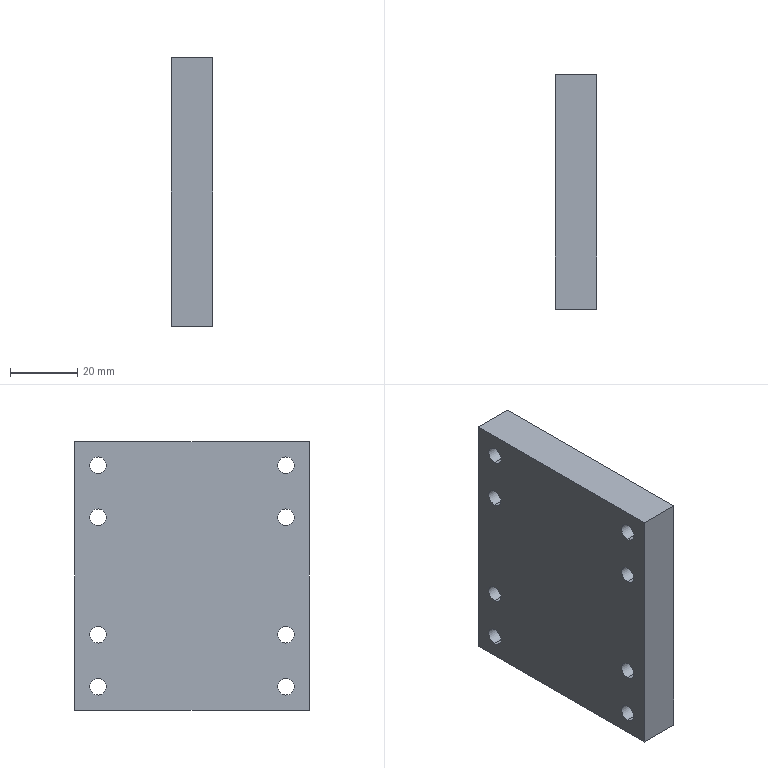Part | SolidWorks | features HoleWzd 2, Extrusion 1 | 1 solid | 22 faces | box 12.4 x 70 x 80 mm | volume 67492 mm3 | cylinder 16 | plane 6 | commonest cylinder face diameters 5 x16
STEP:
#1=CARTESIAN_POINT('',(0.,28.,35.5));
#2=VERTEX_POINT('',#1);
#3=CARTESIAN_POINT('',(0.,28.,30.5));
#4=VERTEX_POINT('',#3);
#5=CARTESIAN_POINT('',(0.,28.,33.));
#6=DIRECTION('',(1.,0.,0.));
#7=DIRECTION('',(0.,0.,-1.));
#8=AXIS2_PLACEMENT_3D('',#5,#6,#7);
#9=CIRCLE('',#8,2.5);
#10=EDGE_CURVE('',#2,#4,#9,.T.);
#11=ORIENTED_EDGE('',*,*,#10,.F.);
#12=CARTESIAN_POINT('',(12.4,28.,35.5));
#13=VERTEX_POINT('',#12);
#14=CARTESIAN_POINT('',(12.4,28.,35.5));
#15=DIRECTION('',(1.,0.,0.));
#16=VECTOR('',#15,1000.);
#17=LINE('',#14,#16);
#18=EDGE_CURVE('',#2,#13,#17,.T.);
#19=ORIENTED_EDGE('',*,*,#18,.T.);
#20=CARTESIAN_POINT('',(12.4,28.,30.5));
#21=VERTEX_POINT('',#20);
#22=CARTESIAN_POINT('',(12.4,28.,33.));
#23=DIRECTION('',(1.,0.,0.));
#24=DIRECTION('',(0.,0.,-1.));
#25=AXIS2_PLACEMENT_3D('',#22,#23,#24);
#26=CIRCLE('',#25,2.5);
#27=EDGE_CURVE('',#13,#21,#26,.T.);
#28=ORIENTED_EDGE('',*,*,#27,.T.);
#29=CARTESIAN_POINT('',(12.4,28.,30.5));
#30=DIRECTION('',(1.,0.,0.));
#31=VECTOR('',#30,1000.);
#32=LINE('',#29,#31);
#33=EDGE_CURVE('',#4,#21,#32,.T.);
#34=ORIENTED_EDGE('',*,*,#33,.F.);
#35=EDGE_LOOP('',(#11,#19,#28,#34));
#36=FACE_OUTER_BOUND('',#35,.T.);
#37=CARTESIAN_POINT('',(12.4,28.,33.));
#38=DIRECTION('',(1.,0.,0.));
#39=DIRECTION('',(0.,0.,-1.));
#40=AXIS2_PLACEMENT_3D('',#37,#38,#39);
#41=CYLINDRICAL_SURFACE('',#40,2.5);
#42=ADVANCED_FACE('',(#36),#41,.F.);
#43=CARTESIAN_POINT('',(0.,-28.,35.5));
#44=VERTEX_POINT('',#43);
#45=CARTESIAN_POINT('',(0.,-28.,30.5));
#46=VERTEX_POINT('',#45);
#47=CARTESIAN_POINT('',(0.,-28.,33.));
#48=DIRECTION('',(1.,0.,0.));
#49=DIRECTION('',(0.,0.,-1.));
#50=AXIS2_PLACEMENT_3D('',#47,#48,#49);
#51=CIRCLE('',#50,2.5);
#52=EDGE_CURVE('',#44,#46,#51,.T.);
#53=ORIENTED_EDGE('',*,*,#52,.F.);
#54=CARTESIAN_POINT('',(12.4,-28.,35.5));
#55=VERTEX_POINT('',#54);
#56=CARTESIAN_POINT('',(12.4,-28.,35.5));
#57=DIRECTION('',(1.,0.,0.));
#58=VECTOR('',#57,1000.);
#59=LINE('',#56,#58);
#60=EDGE_CURVE('',#44,#55,#59,.T.);
#61=ORIENTED_EDGE('',*,*,#60,.T.);
#62=CARTESIAN_POINT('',(12.4,-28.,30.5));
#63=VERTEX_POINT('',#62);
#64=CARTESIAN_POINT('',(12.4,-28.,33.));
#65=DIRECTION('',(1.,0.,0.));
#66=DIRECTION('',(0.,0.,-1.));
#67=AXIS2_PLACEMENT_3D('',#64,#65,#66);
#68=CIRCLE('',#67,2.5);
#69=EDGE_CURVE('',#55,#63,#68,.T.);
#70=ORIENTED_EDGE('',*,*,#69,.T.);
#71=CARTESIAN_POINT('',(12.4,-28.,30.5));
#72=DIRECTION('',(1.,0.,0.));
#73=VECTOR('',#72,1000.);
#74=LINE('',#71,#73);
#75=EDGE_CURVE('',#46,#63,#74,.T.);
#76=ORIENTED_EDGE('',*,*,#75,.F.);
#77=EDGE_LOOP('',(#53,#61,#70,#76));
#78=FACE_OUTER_BOUND('',#77,.T.);
#79=CARTESIAN_POINT('',(12.4,-28.,33.));
#80=DIRECTION('',(1.,0.,0.));
#81=DIRECTION('',(0.,0.,-1.));
#82=AXIS2_PLACEMENT_3D('',#79,#80,#81);
#83=CYLINDRICAL_SURFACE('',#82,2.5);
#84=ADVANCED_FACE('',(#78),#83,.F.);
#85=CARTESIAN_POINT('',(0.,-28.,-30.5));
#86=VERTEX_POINT('',#85);
#87=CARTESIAN_POINT('',(0.,-28.,-35.5));
#88=VERTEX_POINT('',#87);
#89=CARTESIAN_POINT('',(0.,-28.,-33.));
#90=DIRECTION('',(1.,0.,0.));
#91=DIRECTION('',(0.,0.,-1.));
#92=AXIS2_PLACEMENT_3D('',#89,#90,#91);
#93=CIRCLE('',#92,2.5);
#94=EDGE_CURVE('',#86,#88,#93,.T.);
#95=ORIENTED_EDGE('',*,*,#94,.F.);
#96=CARTESIAN_POINT('',(12.4,-28.,-30.5));
#97=VERTEX_POINT('',#96);
#98=CARTESIAN_POINT('',(12.4,-28.,-30.5));
#99=DIRECTION('',(1.,0.,0.));
#100=VECTOR('',#99,1000.);
#101=LINE('',#98,#100);
#102=EDGE_CURVE('',#86,#97,#101,.T.);
#103=ORIENTED_EDGE('',*,*,#102,.T.);
#104=CARTESIAN_POINT('',(12.4,-28.,-35.5));
#105=VERTEX_POINT('',#104);
#106=CARTESIAN_POINT('',(12.4,-28.,-33.));
#107=DIRECTION('',(1.,0.,0.));
#108=DIRECTION('',(0.,0.,-1.));
#109=AXIS2_PLACEMENT_3D('',#106,#107,#108);
#110=CIRCLE('',#109,2.5);
#111=EDGE_CURVE('',#97,#105,#110,.T.);
#112=ORIENTED_EDGE('',*,*,#111,.T.);
#113=CARTESIAN_POINT('',(12.4,-28.,-35.5));
#114=DIRECTION('',(1.,0.,0.));
#115=VECTOR('',#114,1000.);
#116=LINE('',#113,#115);
#117=EDGE_CURVE('',#88,#105,#116,.T.);
#118=ORIENTED_EDGE('',*,*,#117,.F.);
#119=EDGE_LOOP('',(#95,#103,#112,#118));
#120=FACE_OUTER_BOUND('',#119,.T.);
#121=CARTESIAN_POINT('',(12.4,-28.,-33.));
#122=DIRECTION('',(1.,0.,0.));
#123=DIRECTION('',(0.,0.,-1.));
#124=AXIS2_PLACEMENT_3D('',#121,#122,#123);
#125=CYLINDRICAL_SURFACE('',#124,2.5);
#126=ADVANCED_FACE('',(#120),#125,.F.);
#127=CARTESIAN_POINT('',(0.,28.,-30.5));
#128=VERTEX_POINT('',#127);
#129=CARTESIAN_POINT('',(0.,28.,-35.5));
#130=VERTEX_POINT('',#129);
#131=CARTESIAN_POINT('',(0.,28.,-33.));
#132=DIRECTION('',(1.,0.,0.));
#133=DIRECTION('',(0.,0.,-1.));
#134=AXIS2_PLACEMENT_3D('',#131,#132,#133);
#135=CIRCLE('',#134,2.5);
#136=EDGE_CURVE('',#128,#130,#135,.T.);
#137=ORIENTED_EDGE('',*,*,#136,.F.);
#138=CARTESIAN_POINT('',(12.4,28.,-30.5));
#139=VERTEX_POINT('',#138);
#140=CARTESIAN_POINT('',(12.4,28.,-30.5));
#141=DIRECTION('',(1.,0.,0.));
#142=VECTOR('',#141,1000.);
#143=LINE('',#140,#142);
#144=EDGE_CURVE('',#128,#139,#143,.T.);
#145=ORIENTED_EDGE('',*,*,#144,.T.);
#146=CARTESIAN_POINT('',(12.4,28.,-35.5));
#147=VERTEX_POINT('',#146);
#148=CARTESIAN_POINT('',(12.4,28.,-33.));
#149=DIRECTION('',(1.,0.,0.));
#150=DIRECTION('',(0.,0.,-1.));
#151=AXIS2_PLACEMENT_3D('',#148,#149,#150);
#152=CIRCLE('',#151,2.5);
#153=EDGE_CURVE('',#139,#147,#152,.T.);
#154=ORIENTED_EDGE('',*,*,#153,.T.);
#155=CARTESIAN_POINT('',(12.4,28.,-35.5));
#156=DIRECTION('',(1.,0.,0.));
#157=VECTOR('',#156,1000.);
#158=LINE('',#155,#157);
#159=EDGE_CURVE('',#130,#147,#158,.T.);
#160=ORIENTED_EDGE('',*,*,#159,.F.);
#161=EDGE_LOOP('',(#137,#145,#154,#160));
#162=FACE_OUTER_BOUND('',#161,.T.);
#163=CARTESIAN_POINT('',(12.4,28.,-33.));
#164=DIRECTION('',(1.,0.,0.));
#165=DIRECTION('',(0.,0.,-1.));
#166=AXIS2_PLACEMENT_3D('',#163,#164,#165);
#167=CYLINDRICAL_SURFACE('',#166,2.5);
#168=ADVANCED_FACE('',(#162),#167,.F.);
#169=CARTESIAN_POINT('',(0.,28.,20.));
#170=VERTEX_POINT('',#169);
#171=CARTESIAN_POINT('',(0.,28.,15.));
#172=VERTEX_POINT('',#171);
#173=CARTESIAN_POINT('',(0.,28.,17.5));
#174=DIRECTION('',(1.,0.,0.));
#175=DIRECTION('',(0.,0.,-1.));
#176=AXIS2_PLACEMENT_3D('',#173,#174,#175);
#177=CIRCLE('',#176,2.5);
#178=EDGE_CURVE('',#170,#172,#177,.T.);
#179=ORIENTED_EDGE('',*,*,#178,.F.);
#180=CARTESIAN_POINT('',(12.4,28.,20.));
#181=VERTEX_POINT('',#180);
#182=CARTESIAN_POINT('',(12.4,28.,20.));
#183=DIRECTION('',(1.,0.,0.));
#184=VECTOR('',#183,1000.);
#185=LINE('',#182,#184);
#186=EDGE_CURVE('',#170,#181,#185,.T.);
#187=ORIENTED_EDGE('',*,*,#186,.T.);
#188=CARTESIAN_POINT('',(12.4,28.,15.));
#189=VERTEX_POINT('',#188);
#190=CARTESIAN_POINT('',(12.4,28.,17.5));
#191=DIRECTION('',(1.,0.,0.));
#192=DIRECTION('',(0.,0.,-1.));
#193=AXIS2_PLACEMENT_3D('',#190,#191,#192);
#194=CIRCLE('',#193,2.5);
#195=EDGE_CURVE('',#181,#189,#194,.T.);
#196=ORIENTED_EDGE('',*,*,#195,.T.);
#197=CARTESIAN_POINT('',(12.4,28.,15.));
#198=DIRECTION('',(1.,0.,0.));
#199=VECTOR('',#198,1000.);
#200=LINE('',#197,#199);
#201=EDGE_CURVE('',#172,#189,#200,.T.);
#202=ORIENTED_EDGE('',*,*,#201,.F.);
#203=EDGE_LOOP('',(#179,#187,#196,#202));
#204=FACE_OUTER_BOUND('',#203,.T.);
#205=CARTESIAN_POINT('',(12.4,28.,17.5));
#206=DIRECTION('',(1.,0.,0.));
#207=DIRECTION('',(0.,0.,-1.));
#208=AXIS2_PLACEMENT_3D('',#205,#206,#207);
#209=CYLINDRICAL_SURFACE('',#208,2.5);
#210=ADVANCED_FACE('',(#204),#209,.F.);
#211=CARTESIAN_POINT('',(0.,28.,-15.));
#212=VERTEX_POINT('',#211);
#213=CARTESIAN_POINT('',(0.,28.,-20.));
#214=VERTEX_POINT('',#213);
#215=CARTESIAN_POINT('',(0.,28.,-17.5));
#216=DIRECTION('',(1.,0.,0.));
#217=DIRECTION('',(0.,0.,-1.));
#218=AXIS2_PLACEMENT_3D('',#215,#216,#217);
#219=CIRCLE('',#218,2.5);
#220=EDGE_CURVE('',#212,#214,#219,.T.);
#221=ORIENTED_EDGE('',*,*,#220,.F.);
#222=CARTESIAN_POINT('',(12.4,28.,-15.));
#223=VERTEX_POINT('',#222);
#224=CARTESIAN_POINT('',(12.4,28.,-15.));
#225=DIRECTION('',(1.,0.,0.));
#226=VECTOR('',#225,1000.);
#227=LINE('',#224,#226);
#228=EDGE_CURVE('',#212,#223,#227,.T.);
#229=ORIENTED_EDGE('',*,*,#228,.T.);
#230=CARTESIAN_POINT('',(12.4,28.,-20.));
#231=VERTEX_POINT('',#230);
#232=CARTESIAN_POINT('',(12.4,28.,-17.5));
#233=DIRECTION('',(1.,0.,0.));
#234=DIRECTION('',(0.,0.,-1.));
#235=AXIS2_PLACEMENT_3D('',#232,#233,#234);
#236=CIRCLE('',#235,2.5);
#237=EDGE_CURVE('',#223,#231,#236,.T.);
#238=ORIENTED_EDGE('',*,*,#237,.T.);
#239=CARTESIAN_POINT('',(12.4,28.,-20.));
#240=DIRECTION('',(1.,0.,0.));
#241=VECTOR('',#240,1000.);
#242=LINE('',#239,#241);
#243=EDGE_CURVE('',#214,#231,#242,.T.);
#244=ORIENTED_EDGE('',*,*,#243,.F.);
#245=EDGE_LOOP('',(#221,#229,#238,#244));
#246=FACE_OUTER_BOUND('',#245,.T.);
#247=CARTESIAN_POINT('',(12.4,28.,-17.5));
#248=DIRECTION('',(1.,0.,0.));
#249=DIRECTION('',(0.,0.,-1.));
#250=AXIS2_PLACEMENT_3D('',#247,#248,#249);
#251=CYLINDRICAL_SURFACE('',#250,2.5);
#252=ADVANCED_FACE('',(#246),#251,.F.);
#253=CARTESIAN_POINT('',(0.,-28.,20.));
#254=VERTEX_POINT('',#253);
#255=CARTESIAN_POINT('',(0.,-28.,15.));
#256=VERTEX_POINT('',#255);
#257=CARTESIAN_POINT('',(0.,-28.,17.5));
#258=DIRECTION('',(1.,0.,0.));
#259=DIRECTION('',(0.,0.,-1.));
#260=AXIS2_PLACEMENT_3D('',#257,#258,#259);
#261=CIRCLE('',#260,2.5);
#262=EDGE_CURVE('',#254,#256,#261,.T.);
#263=ORIENTED_EDGE('',*,*,#262,.F.);
#264=CARTESIAN_POINT('',(12.4,-28.,20.));
#265=VERTEX_POINT('',#264);
#266=CARTESIAN_POINT('',(12.4,-28.,20.));
#267=DIRECTION('',(1.,0.,0.));
#268=VECTOR('',#267,1000.);
#269=LINE('',#266,#268);
#270=EDGE_CURVE('',#254,#265,#269,.T.);
#271=ORIENTED_EDGE('',*,*,#270,.T.);
#272=CARTESIAN_POINT('',(12.4,-28.,15.));
#273=VERTEX_POINT('',#272);
#274=CARTESIAN_POINT('',(12.4,-28.,17.5));
#275=DIRECTION('',(1.,0.,0.));
#276=DIRECTION('',(0.,0.,-1.));
#277=AXIS2_PLACEMENT_3D('',#274,#275,#276);
#278=CIRCLE('',#277,2.5);
#279=EDGE_CURVE('',#265,#273,#278,.T.);
#280=ORIENTED_EDGE('',*,*,#279,.T.);
#281=CARTESIAN_POINT('',(12.4,-28.,15.));
#282=DIRECTION('',(1.,0.,0.));
#283=VECTOR('',#282,1000.);
#284=LINE('',#281,#283);
#285=EDGE_CURVE('',#256,#273,#284,.T.);
#286=ORIENTED_EDGE('',*,*,#285,.F.);
#287=EDGE_LOOP('',(#263,#271,#280,#286));
#288=FACE_OUTER_BOUND('',#287,.T.);
#289=CARTESIAN_POINT('',(12.4,-28.,17.5));
#290=DIRECTION('',(1.,0.,0.));
#291=DIRECTION('',(0.,0.,-1.));
#292=AXIS2_PLACEMENT_3D('',#289,#290,#291);
#293=CYLINDRICAL_SURFACE('',#292,2.5);
#294=ADVANCED_FACE('',(#288),#293,.F.);
#295=CARTESIAN_POINT('',(0.,-28.,-15.));
#296=VERTEX_POINT('',#295);
#297=CARTESIAN_POINT('',(0.,-28.,-20.));
#298=VERTEX_POINT('',#297);
#299=CARTESIAN_POINT('',(0.,-28.,-17.5));
#300=DIRECTION('',(1.,0.,0.));
#301=DIRECTION('',(0.,0.,-1.));
#302=AXIS2_PLACEMENT_3D('',#299,#300,#301);
#303=CIRCLE('',#302,2.5);
#304=EDGE_CURVE('',#296,#298,#303,.T.);
#305=ORIENTED_EDGE('',*,*,#304,.F.);
#306=CARTESIAN_POINT('',(12.4,-28.,-15.));
#307=VERTEX_POINT('',#306);
#308=CARTESIAN_POINT('',(12.4,-28.,-15.));
#309=DIRECTION('',(1.,0.,0.));
#310=VECTOR('',#309,1000.);
#311=LINE('',#308,#310);
#312=EDGE_CURVE('',#296,#307,#311,.T.);
#313=ORIENTED_EDGE('',*,*,#312,.T.);
#314=CARTESIAN_POINT('',(12.4,-28.,-20.));
#315=VERTEX_POINT('',#314);
#316=CARTESIAN_POINT('',(12.4,-28.,-17.5));
#317=DIRECTION('',(1.,0.,0.));
#318=DIRECTION('',(0.,0.,-1.));
#319=AXIS2_PLACEMENT_3D('',#316,#317,#318);
#320=CIRCLE('',#319,2.5);
#321=EDGE_CURVE('',#307,#315,#320,.T.);
#322=ORIENTED_EDGE('',*,*,#321,.T.);
#323=CARTESIAN_POINT('',(12.4,-28.,-20.));
#324=DIRECTION('',(1.,0.,0.));
#325=VECTOR('',#324,1000.);
#326=LINE('',#323,#325);
#327=EDGE_CURVE('',#298,#315,#326,.T.);
#328=ORIENTED_EDGE('',*,*,#327,.F.);
#329=EDGE_LOOP('',(#305,#313,#322,#328));
#330=FACE_OUTER_BOUND('',#329,.T.);
#331=CARTESIAN_POINT('',(12.4,-28.,-17.5));
#332=DIRECTION('',(1.,0.,0.));
#333=DIRECTION('',(0.,0.,-1.));
#334=AXIS2_PLACEMENT_3D('',#331,#332,#333);
#335=CYLINDRICAL_SURFACE('',#334,2.5);
#336=ADVANCED_FACE('',(#330),#335,.F.);
#337=CARTESIAN_POINT('',(0.,-35.,-40.));
#338=VERTEX_POINT('',#337);
#339=CARTESIAN_POINT('',(0.,35.,-40.));
#340=VERTEX_POINT('',#339);
#341=CARTESIAN_POINT('',(0.,35.,-40.));
#342=DIRECTION('',(0.,1.,0.));
#343=VECTOR('',#342,1000.);
#344=LINE('',#341,#343);
#345=EDGE_CURVE('',#338,#340,#344,.T.);
#346=ORIENTED_EDGE('',*,*,#345,.T.);
#347=CARTESIAN_POINT('',(12.4,35.,-40.));
#348=VERTEX_POINT('',#347);
#349=CARTESIAN_POINT('',(12.4,35.,-40.));
#350=DIRECTION('',(-1.,0.,0.));
#351=VECTOR('',#350,1000.);
#352=LINE('',#349,#351);
#353=EDGE_CURVE('',#348,#340,#352,.T.);
#354=ORIENTED_EDGE('',*,*,#353,.F.);
#355=CARTESIAN_POINT('',(12.4,-35.,-40.));
#356=VERTEX_POINT('',#355);
#357=CARTESIAN_POINT('',(12.4,35.,-40.));
#358=DIRECTION('',(0.,1.,0.));
#359=VECTOR('',#358,1000.);
#360=LINE('',#357,#359);
#361=EDGE_CURVE('',#356,#348,#360,.T.);
#362=ORIENTED_EDGE('',*,*,#361,.F.);
#363=CARTESIAN_POINT('',(12.4,-35.,-40.));
#364=DIRECTION('',(-1.,0.,0.));
#365=VECTOR('',#364,1000.);
#366=LINE('',#363,#365);
#367=EDGE_CURVE('',#356,#338,#366,.T.);
#368=ORIENTED_EDGE('',*,*,#367,.T.);
#369=EDGE_LOOP('',(#346,#354,#362,#368));
#370=FACE_OUTER_BOUND('',#369,.T.);
#371=CARTESIAN_POINT('',(12.4,35.,-40.));
#372=DIRECTION('',(0.,0.,1.));
#373=DIRECTION('',(0.,-1.,0.));
#374=AXIS2_PLACEMENT_3D('',#371,#372,#373);
#375=PLANE('',#374);
#376=ADVANCED_FACE('',(#370),#375,.F.);
#377=CARTESIAN_POINT('',(0.,35.,40.));
#378=VERTEX_POINT('',#377);
#379=CARTESIAN_POINT('',(0.,35.,40.));
#380=DIRECTION('',(0.,0.,1.));
#381=VECTOR('',#380,1000.);
#382=LINE('',#379,#381);
#383=EDGE_CURVE('',#340,#378,#382,.T.);
#384=ORIENTED_EDGE('',*,*,#383,.T.);
#385=CARTESIAN_POINT('',(12.4,35.,40.));
#386=VERTEX_POINT('',#385);
#387=CARTESIAN_POINT('',(12.4,35.,40.));
#388=DIRECTION('',(-1.,0.,0.));
#389=VECTOR('',#388,1000.);
#390=LINE('',#387,#389);
#391=EDGE_CURVE('',#386,#378,#390,.T.);
#392=ORIENTED_EDGE('',*,*,#391,.F.);
#393=CARTESIAN_POINT('',(12.4,35.,40.));
#394=DIRECTION('',(0.,0.,1.));
#395=VECTOR('',#394,1000.);
#396=LINE('',#393,#395);
#397=EDGE_CURVE('',#348,#386,#396,.T.);
#398=ORIENTED_EDGE('',*,*,#397,.F.);
#399=ORIENTED_EDGE('',*,*,#353,.T.);
#400=EDGE_LOOP('',(#384,#392,#398,#399));
#401=FACE_OUTER_BOUND('',#400,.T.);
#402=CARTESIAN_POINT('',(12.4,35.,40.));
#403=DIRECTION('',(0.,-1.,0.));
#404=DIRECTION('',(0.,0.,-1.));
#405=AXIS2_PLACEMENT_3D('',#402,#403,#404);
#406=PLANE('',#405);
#407=ADVANCED_FACE('',(#401),#406,.F.);
#408=CARTESIAN_POINT('',(0.,-35.,40.));
#409=VERTEX_POINT('',#408);
#410=CARTESIAN_POINT('',(0.,35.,40.));
#411=DIRECTION('',(0.,-1.,0.));
#412=VECTOR('',#411,1000.);
#413=LINE('',#410,#412);
#414=EDGE_CURVE('',#378,#409,#413,.T.);
#415=ORIENTED_EDGE('',*,*,#414,.T.);
#416=CARTESIAN_POINT('',(12.4,-35.,40.));
#417=VERTEX_POINT('',#416);
#418=CARTESIAN_POINT('',(12.4,-35.,40.));
#419=DIRECTION('',(-1.,0.,0.));
#420=VECTOR('',#419,1000.);
#421=LINE('',#418,#420);
#422=EDGE_CURVE('',#417,#409,#421,.T.);
#423=ORIENTED_EDGE('',*,*,#422,.F.);
#424=CARTESIAN_POINT('',(12.4,35.,40.));
#425=DIRECTION('',(0.,-1.,0.));
#426=VECTOR('',#425,1000.);
#427=LINE('',#424,#426);
#428=EDGE_CURVE('',#386,#417,#427,.T.);
#429=ORIENTED_EDGE('',*,*,#428,.F.);
#430=ORIENTED_EDGE('',*,*,#391,.T.);
#431=EDGE_LOOP('',(#415,#423,#429,#430));
#432=FACE_OUTER_BOUND('',#431,.T.);
#433=CARTESIAN_POINT('',(12.4,35.,40.));
#434=DIRECTION('',(0.,0.,-1.));
#435=DIRECTION('',(0.,1.,0.));
#436=AXIS2_PLACEMENT_3D('',#433,#434,#435);
#437=PLANE('',#436);
#438=ADVANCED_FACE('',(#432),#437,.F.);
#439=CARTESIAN_POINT('',(0.,-35.,40.));
#440=DIRECTION('',(0.,0.,-1.));
#441=VECTOR('',#440,1000.);
#442=LINE('',#439,#441);
#443=EDGE_CURVE('',#409,#338,#442,.T.);
#444=ORIENTED_EDGE('',*,*,#443,.T.);
#445=ORIENTED_EDGE('',*,*,#367,.F.);
#446=CARTESIAN_POINT('',(12.4,-35.,40.));
#447=DIRECTION('',(0.,0.,-1.));
#448=VECTOR('',#447,1000.);
#449=LINE('',#446,#448);
#450=EDGE_CURVE('',#417,#356,#449,.T.);
#451=ORIENTED_EDGE('',*,*,#450,.F.);
#452=ORIENTED_EDGE('',*,*,#422,.T.);
#453=EDGE_LOOP('',(#444,#445,#451,#452));
#454=FACE_OUTER_BOUND('',#453,.T.);
#455=CARTESIAN_POINT('',(12.4,-35.,40.));
#456=DIRECTION('',(0.,1.,0.));
#457=DIRECTION('',(0.,0.,1.));
#458=AXIS2_PLACEMENT_3D('',#455,#456,#457);
#459=PLANE('',#458);
#460=ADVANCED_FACE('',(#454),#459,.F.);
#461=CARTESIAN_POINT('',(12.4,28.,33.));
#462=DIRECTION('',(1.,0.,0.));
#463=DIRECTION('',(0.,0.,-1.));
#464=AXIS2_PLACEMENT_3D('',#461,#462,#463);
#465=CIRCLE('',#464,2.5);
#466=EDGE_CURVE('',#21,#13,#465,.T.);
#467=ORIENTED_EDGE('',*,*,#466,.F.);
#468=ORIENTED_EDGE('',*,*,#27,.F.);
#469=EDGE_LOOP('',(#467,#468));
#470=FACE_BOUND('',#469,.T.);
#471=CARTESIAN_POINT('',(12.4,-28.,33.));
#472=DIRECTION('',(1.,0.,0.));
#473=DIRECTION('',(0.,0.,-1.));
#474=AXIS2_PLACEMENT_3D('',#471,#472,#473);
#475=CIRCLE('',#474,2.5);
#476=EDGE_CURVE('',#63,#55,#475,.T.);
#477=ORIENTED_EDGE('',*,*,#476,.F.);
#478=ORIENTED_EDGE('',*,*,#69,.F.);
#479=EDGE_LOOP('',(#477,#478));
#480=FACE_BOUND('',#479,.T.);
#481=CARTESIAN_POINT('',(12.4,-28.,-33.));
#482=DIRECTION('',(1.,0.,0.));
#483=DIRECTION('',(0.,0.,-1.));
#484=AXIS2_PLACEMENT_3D('',#481,#482,#483);
#485=CIRCLE('',#484,2.5);
#486=EDGE_CURVE('',#105,#97,#485,.T.);
#487=ORIENTED_EDGE('',*,*,#486,.F.);
#488=ORIENTED_EDGE('',*,*,#111,.F.);
#489=EDGE_LOOP('',(#487,#488));
#490=FACE_BOUND('',#489,.T.);
#491=CARTESIAN_POINT('',(12.4,28.,-33.));
#492=DIRECTION('',(1.,0.,0.));
#493=DIRECTION('',(0.,0.,-1.));
#494=AXIS2_PLACEMENT_3D('',#491,#492,#493);
#495=CIRCLE('',#494,2.5);
#496=EDGE_CURVE('',#147,#139,#495,.T.);
#497=ORIENTED_EDGE('',*,*,#496,.F.);
#498=ORIENTED_EDGE('',*,*,#153,.F.);
#499=EDGE_LOOP('',(#497,#498));
#500=FACE_BOUND('',#499,.T.);
#501=CARTESIAN_POINT('',(12.4,28.,17.5));
#502=DIRECTION('',(1.,0.,0.));
#503=DIRECTION('',(0.,0.,-1.));
#504=AXIS2_PLACEMENT_3D('',#501,#502,#503);
#505=CIRCLE('',#504,2.5);
#506=EDGE_CURVE('',#189,#181,#505,.T.);
#507=ORIENTED_EDGE('',*,*,#506,.F.);
#508=ORIENTED_EDGE('',*,*,#195,.F.);
#509=EDGE_LOOP('',(#507,#508));
#510=FACE_BOUND('',#509,.T.);
#511=CARTESIAN_POINT('',(12.4,28.,-17.5));
#512=DIRECTION('',(1.,0.,0.));
#513=DIRECTION('',(0.,0.,-1.));
#514=AXIS2_PLACEMENT_3D('',#511,#512,#513);
#515=CIRCLE('',#514,2.5);
#516=EDGE_CURVE('',#231,#223,#515,.T.);
#517=ORIENTED_EDGE('',*,*,#516,.F.);
#518=ORIENTED_EDGE('',*,*,#237,.F.);
#519=EDGE_LOOP('',(#517,#518));
#520=FACE_BOUND('',#519,.T.);
#521=CARTESIAN_POINT('',(12.4,-28.,17.5));
#522=DIRECTION('',(1.,0.,0.));
#523=DIRECTION('',(0.,0.,-1.));
#524=AXIS2_PLACEMENT_3D('',#521,#522,#523);
#525=CIRCLE('',#524,2.5);
#526=EDGE_CURVE('',#273,#265,#525,.T.);
#527=ORIENTED_EDGE('',*,*,#526,.F.);
#528=ORIENTED_EDGE('',*,*,#279,.F.);
#529=EDGE_LOOP('',(#527,#528));
#530=FACE_BOUND('',#529,.T.);
#531=CARTESIAN_POINT('',(12.4,-28.,-17.5));
#532=DIRECTION('',(1.,0.,0.));
#533=DIRECTION('',(0.,0.,-1.));
#534=AXIS2_PLACEMENT_3D('',#531,#532,#533);
#535=CIRCLE('',#534,2.5);
#536=EDGE_CURVE('',#315,#307,#535,.T.);
#537=ORIENTED_EDGE('',*,*,#536,.F.);
#538=ORIENTED_EDGE('',*,*,#321,.F.);
#539=EDGE_LOOP('',(#537,#538));
#540=FACE_BOUND('',#539,.T.);
#541=ORIENTED_EDGE('',*,*,#361,.T.);
#542=ORIENTED_EDGE('',*,*,#397,.T.);
#543=ORIENTED_EDGE('',*,*,#428,.T.);
#544=ORIENTED_EDGE('',*,*,#450,.T.);
#545=EDGE_LOOP('',(#541,#542,#543,#544));
#546=FACE_OUTER_BOUND('',#545,.T.);
#547=CARTESIAN_POINT('',(12.4,0.,0.));
#548=DIRECTION('',(1.,0.,0.));
#549=DIRECTION('',(0.,0.,-1.));
#550=AXIS2_PLACEMENT_3D('',#547,#548,#549);
#551=PLANE('',#550);
#552=ADVANCED_FACE('',(#470,#480,#490,#500,#510,#520,#530,#540,#546),#551,.T.);
#553=CARTESIAN_POINT('',(0.,28.,33.));
#554=DIRECTION('',(1.,0.,0.));
#555=DIRECTION('',(0.,0.,-1.));
#556=AXIS2_PLACEMENT_3D('',#553,#554,#555);
#557=CIRCLE('',#556,2.5);
#558=EDGE_CURVE('',#4,#2,#557,.T.);
#559=ORIENTED_EDGE('',*,*,#558,.T.);
#560=ORIENTED_EDGE('',*,*,#10,.T.);
#561=EDGE_LOOP('',(#559,#560));
#562=FACE_BOUND('',#561,.T.);
#563=CARTESIAN_POINT('',(0.,-28.,33.));
#564=DIRECTION('',(1.,0.,0.));
#565=DIRECTION('',(0.,0.,-1.));
#566=AXIS2_PLACEMENT_3D('',#563,#564,#565);
#567=CIRCLE('',#566,2.5);
#568=EDGE_CURVE('',#46,#44,#567,.T.);
#569=ORIENTED_EDGE('',*,*,#568,.T.);
#570=ORIENTED_EDGE('',*,*,#52,.T.);
#571=EDGE_LOOP('',(#569,#570));
#572=FACE_BOUND('',#571,.T.);
#573=CARTESIAN_POINT('',(0.,-28.,-33.));
#574=DIRECTION('',(1.,0.,0.));
#575=DIRECTION('',(0.,0.,-1.));
#576=AXIS2_PLACEMENT_3D('',#573,#574,#575);
#577=CIRCLE('',#576,2.5);
#578=EDGE_CURVE('',#88,#86,#577,.T.);
#579=ORIENTED_EDGE('',*,*,#578,.T.);
#580=ORIENTED_EDGE('',*,*,#94,.T.);
#581=EDGE_LOOP('',(#579,#580));
#582=FACE_BOUND('',#581,.T.);
#583=CARTESIAN_POINT('',(0.,28.,-33.));
#584=DIRECTION('',(1.,0.,0.));
#585=DIRECTION('',(0.,0.,-1.));
#586=AXIS2_PLACEMENT_3D('',#583,#584,#585);
#587=CIRCLE('',#586,2.5);
#588=EDGE_CURVE('',#130,#128,#587,.T.);
#589=ORIENTED_EDGE('',*,*,#588,.T.);
#590=ORIENTED_EDGE('',*,*,#136,.T.);
#591=EDGE_LOOP('',(#589,#590));
#592=FACE_BOUND('',#591,.T.);
#593=CARTESIAN_POINT('',(0.,28.,17.5));
#594=DIRECTION('',(1.,0.,0.));
#595=DIRECTION('',(0.,0.,-1.));
#596=AXIS2_PLACEMENT_3D('',#593,#594,#595);
#597=CIRCLE('',#596,2.5);
#598=EDGE_CURVE('',#172,#170,#597,.T.);
#599=ORIENTED_EDGE('',*,*,#598,.T.);
#600=ORIENTED_EDGE('',*,*,#178,.T.);
#601=EDGE_LOOP('',(#599,#600));
#602=FACE_BOUND('',#601,.T.);
#603=CARTESIAN_POINT('',(0.,28.,-17.5));
#604=DIRECTION('',(1.,0.,0.));
#605=DIRECTION('',(0.,0.,-1.));
#606=AXIS2_PLACEMENT_3D('',#603,#604,#605);
#607=CIRCLE('',#606,2.5);
#608=EDGE_CURVE('',#214,#212,#607,.T.);
#609=ORIENTED_EDGE('',*,*,#608,.T.);
#610=ORIENTED_EDGE('',*,*,#220,.T.);
#611=EDGE_LOOP('',(#609,#610));
#612=FACE_BOUND('',#611,.T.);
#613=CARTESIAN_POINT('',(0.,-28.,17.5));
#614=DIRECTION('',(1.,0.,0.));
#615=DIRECTION('',(0.,0.,-1.));
#616=AXIS2_PLACEMENT_3D('',#613,#614,#615);
#617=CIRCLE('',#616,2.5);
#618=EDGE_CURVE('',#256,#254,#617,.T.);
#619=ORIENTED_EDGE('',*,*,#618,.T.);
#620=ORIENTED_EDGE('',*,*,#262,.T.);
#621=EDGE_LOOP('',(#619,#620));
#622=FACE_BOUND('',#621,.T.);
#623=CARTESIAN_POINT('',(0.,-28.,-17.5));
#624=DIRECTION('',(1.,0.,0.));
#625=DIRECTION('',(0.,0.,-1.));
#626=AXIS2_PLACEMENT_3D('',#623,#624,#625);
#627=CIRCLE('',#626,2.5);
#628=EDGE_CURVE('',#298,#296,#627,.T.);
#629=ORIENTED_EDGE('',*,*,#628,.T.);
#630=ORIENTED_EDGE('',*,*,#304,.T.);
#631=EDGE_LOOP('',(#629,#630));
#632=FACE_BOUND('',#631,.T.);
#633=ORIENTED_EDGE('',*,*,#345,.F.);
#634=ORIENTED_EDGE('',*,*,#443,.F.);
#635=ORIENTED_EDGE('',*,*,#414,.F.);
#636=ORIENTED_EDGE('',*,*,#383,.F.);
#637=EDGE_LOOP('',(#633,#634,#635,#636));
#638=FACE_OUTER_BOUND('',#637,.T.);
#639=CARTESIAN_POINT('',(0.,0.,0.));
#640=DIRECTION('',(1.,0.,0.));
#641=DIRECTION('',(0.,0.,-1.));
#642=AXIS2_PLACEMENT_3D('',#639,#640,#641);
#643=PLANE('',#642);
#644=ADVANCED_FACE('',(#562,#572,#582,#592,#602,#612,#622,#632,#638),#643,.F.);
#645=ORIENTED_EDGE('',*,*,#312,.F.);
#646=ORIENTED_EDGE('',*,*,#628,.F.);
#647=ORIENTED_EDGE('',*,*,#327,.T.);
#648=ORIENTED_EDGE('',*,*,#536,.T.);
#649=EDGE_LOOP('',(#645,#646,#647,#648));
#650=FACE_OUTER_BOUND('',#649,.T.);
#651=CARTESIAN_POINT('',(12.4,-28.,-17.5));
#652=DIRECTION('',(1.,0.,0.));
#653=DIRECTION('',(0.,0.,-1.));
#654=AXIS2_PLACEMENT_3D('',#651,#652,#653);
#655=CYLINDRICAL_SURFACE('',#654,2.5);
#656=ADVANCED_FACE('',(#650),#655,.F.);
#657=ORIENTED_EDGE('',*,*,#270,.F.);
#658=ORIENTED_EDGE('',*,*,#618,.F.);
#659=ORIENTED_EDGE('',*,*,#285,.T.);
#660=ORIENTED_EDGE('',*,*,#526,.T.);
#661=EDGE_LOOP('',(#657,#658,#659,#660));
#662=FACE_OUTER_BOUND('',#661,.T.);
#663=CARTESIAN_POINT('',(12.4,-28.,17.5));
#664=DIRECTION('',(1.,0.,0.));
#665=DIRECTION('',(0.,0.,-1.));
#666=AXIS2_PLACEMENT_3D('',#663,#664,#665);
#667=CYLINDRICAL_SURFACE('',#666,2.5);
#668=ADVANCED_FACE('',(#662),#667,.F.);
#669=ORIENTED_EDGE('',*,*,#228,.F.);
#670=ORIENTED_EDGE('',*,*,#608,.F.);
#671=ORIENTED_EDGE('',*,*,#243,.T.);
#672=ORIENTED_EDGE('',*,*,#516,.T.);
#673=EDGE_LOOP('',(#669,#670,#671,#672));
#674=FACE_OUTER_BOUND('',#673,.T.);
#675=CARTESIAN_POINT('',(12.4,28.,-17.5));
#676=DIRECTION('',(1.,0.,0.));
#677=DIRECTION('',(0.,0.,-1.));
#678=AXIS2_PLACEMENT_3D('',#675,#676,#677);
#679=CYLINDRICAL_SURFACE('',#678,2.5);
#680=ADVANCED_FACE('',(#674),#679,.F.);
#681=ORIENTED_EDGE('',*,*,#186,.F.);
#682=ORIENTED_EDGE('',*,*,#598,.F.);
#683=ORIENTED_EDGE('',*,*,#201,.T.);
#684=ORIENTED_EDGE('',*,*,#506,.T.);
#685=EDGE_LOOP('',(#681,#682,#683,#684));
#686=FACE_OUTER_BOUND('',#685,.T.);
#687=CARTESIAN_POINT('',(12.4,28.,17.5));
#688=DIRECTION('',(1.,0.,0.));
#689=DIRECTION('',(0.,0.,-1.));
#690=AXIS2_PLACEMENT_3D('',#687,#688,#689);
#691=CYLINDRICAL_SURFACE('',#690,2.5);
#692=ADVANCED_FACE('',(#686),#691,.F.);
#693=ORIENTED_EDGE('',*,*,#144,.F.);
#694=ORIENTED_EDGE('',*,*,#588,.F.);
#695=ORIENTED_EDGE('',*,*,#159,.T.);
#696=ORIENTED_EDGE('',*,*,#496,.T.);
#697=EDGE_LOOP('',(#693,#694,#695,#696));
#698=FACE_OUTER_BOUND('',#697,.T.);
#699=CARTESIAN_POINT('',(12.4,28.,-33.));
#700=DIRECTION('',(1.,0.,0.));
#701=DIRECTION('',(0.,0.,-1.));
#702=AXIS2_PLACEMENT_3D('',#699,#700,#701);
#703=CYLINDRICAL_SURFACE('',#702,2.5);
#704=ADVANCED_FACE('',(#698),#703,.F.);
#705=ORIENTED_EDGE('',*,*,#102,.F.);
#706=ORIENTED_EDGE('',*,*,#578,.F.);
#707=ORIENTED_EDGE('',*,*,#117,.T.);
#708=ORIENTED_EDGE('',*,*,#486,.T.);
#709=EDGE_LOOP('',(#705,#706,#707,#708));
#710=FACE_OUTER_BOUND('',#709,.T.);
#711=CARTESIAN_POINT('',(12.4,-28.,-33.));
#712=DIRECTION('',(1.,0.,0.));
#713=DIRECTION('',(0.,0.,-1.));
#714=AXIS2_PLACEMENT_3D('',#711,#712,#713);
#715=CYLINDRICAL_SURFACE('',#714,2.5);
#716=ADVANCED_FACE('',(#710),#715,.F.);
#717=ORIENTED_EDGE('',*,*,#60,.F.);
#718=ORIENTED_EDGE('',*,*,#568,.F.);
#719=ORIENTED_EDGE('',*,*,#75,.T.);
#720=ORIENTED_EDGE('',*,*,#476,.T.);
#721=EDGE_LOOP('',(#717,#718,#719,#720));
#722=FACE_OUTER_BOUND('',#721,.T.);
#723=CARTESIAN_POINT('',(12.4,-28.,33.));
#724=DIRECTION('',(1.,0.,0.));
#725=DIRECTION('',(0.,0.,-1.));
#726=AXIS2_PLACEMENT_3D('',#723,#724,#725);
#727=CYLINDRICAL_SURFACE('',#726,2.5);
#728=ADVANCED_FACE('',(#722),#727,.F.);
#729=ORIENTED_EDGE('',*,*,#18,.F.);
#730=ORIENTED_EDGE('',*,*,#558,.F.);
#731=ORIENTED_EDGE('',*,*,#33,.T.);
#732=ORIENTED_EDGE('',*,*,#466,.T.);
#733=EDGE_LOOP('',(#729,#730,#731,#732));
#734=FACE_OUTER_BOUND('',#733,.T.);
#735=CARTESIAN_POINT('',(12.4,28.,33.));
#736=DIRECTION('',(1.,0.,0.));
#737=DIRECTION('',(0.,0.,-1.));
#738=AXIS2_PLACEMENT_3D('',#735,#736,#737);
#739=CYLINDRICAL_SURFACE('',#738,2.5);
#740=ADVANCED_FACE('',(#734),#739,.F.);
#741=CLOSED_SHELL('',(#42,#84,#126,#168,#210,#252,#294,#336,#376,#407,#438,#460,#552,#644,#656,#668,#680,#692,#704,#716,#728,#740));
#742=MANIFOLD_SOLID_BREP('',#741);
#743=CARTESIAN_POINT('',(0.,0.,0.));
#744=DIRECTION('',(0.,0.,1.));
#745=DIRECTION('',(1.,0.,0.));
#746=AXIS2_PLACEMENT_3D('',#743,#744,#745);
#747=(LENGTH_UNIT()NAMED_UNIT(*)SI_UNIT(.MILLI.,.METRE.));
#748=UNCERTAINTY_MEASURE_WITH_UNIT(LENGTH_MEASURE(0.00001),#747,'','');
#749=(NAMED_UNIT(*)PLANE_ANGLE_UNIT()SI_UNIT($,.RADIAN.));
#750=(NAMED_UNIT(*)SI_UNIT($,.STERADIAN.)SOLID_ANGLE_UNIT());
#751=(GEOMETRIC_REPRESENTATION_CONTEXT(3)GLOBAL_UNCERTAINTY_ASSIGNED_CONTEXT((#748))GLOBAL_UNIT_ASSIGNED_CONTEXT((#747,#749,#750))REPRESENTATION_CONTEXT('',''));
#752=ADVANCED_BREP_SHAPE_REPRESENTATION('',(#742,#746),#751);